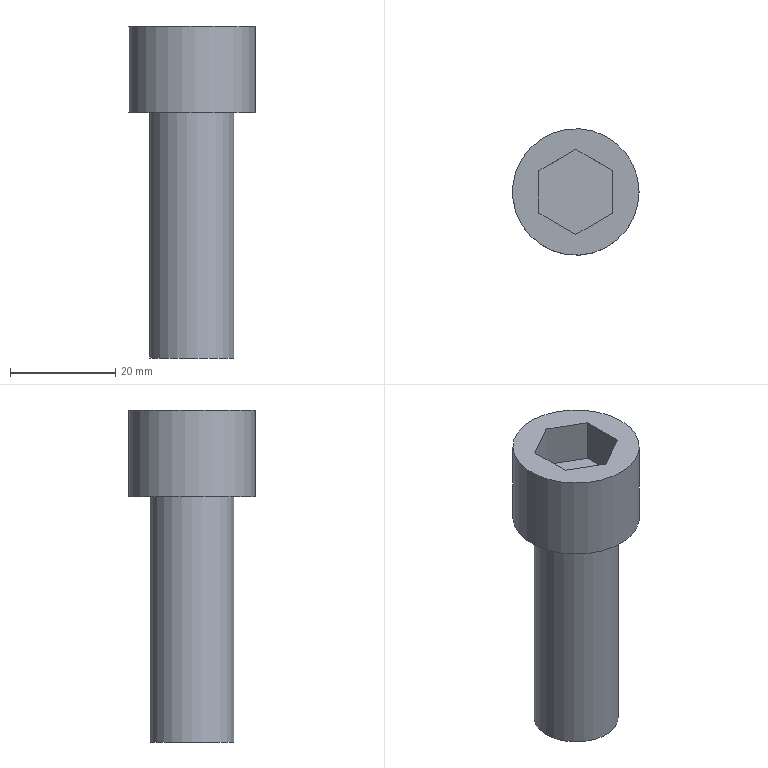Part | NX | features MPPJ 2 | 1 solid | 12 faces | box 24 x 24 x 63 mm | volume 15413 mm3 | plane 10 | cylinder 2 | commonest cylinder face diameters 16 x1 24 x1
STEP:
#1=CARTESIAN_POINT('',(154.5,89.,99.5));
#2=VERTEX_POINT('',#1);
#3=CARTESIAN_POINT('',(142.5,89.,99.5));
#4=DIRECTION('',(0.,0.,-1.));
#5=DIRECTION('',(1.,0.,0.));
#6=AXIS2_PLACEMENT_3D('',#3,#4,#5);
#7=CIRCLE('',#6,12.);
#8=EDGE_CURVE('',#2,#2,#7,.T.);
#9=ORIENTED_EDGE('',*,*,#8,.F.);
#10=EDGE_LOOP('',(#9));
#11=FACE_BOUND('',#10,.T.);
#12=CARTESIAN_POINT('',(149.5,84.959,99.5));
#13=VERTEX_POINT('',#12);
#14=CARTESIAN_POINT('',(142.5,80.917,99.5));
#15=VERTEX_POINT('',#14);
#16=CARTESIAN_POINT('',(149.5,84.959,99.5));
#17=DIRECTION('',(-0.866,-0.5,0.));
#18=VECTOR('',#17,1000.);
#19=LINE('',#16,#18);
#20=EDGE_CURVE('',#13,#15,#19,.T.);
#21=ORIENTED_EDGE('',*,*,#20,.T.);
#22=CARTESIAN_POINT('',(135.5,84.959,99.5));
#23=VERTEX_POINT('',#22);
#24=CARTESIAN_POINT('',(142.5,80.917,99.5));
#25=DIRECTION('',(-0.866,0.5,0.));
#26=VECTOR('',#25,1000.);
#27=LINE('',#24,#26);
#28=EDGE_CURVE('',#15,#23,#27,.T.);
#29=ORIENTED_EDGE('',*,*,#28,.T.);
#30=CARTESIAN_POINT('',(135.5,93.041,99.5));
#31=VERTEX_POINT('',#30);
#32=CARTESIAN_POINT('',(135.5,84.959,99.5));
#33=DIRECTION('',(0.,1.,0.));
#34=VECTOR('',#33,1000.);
#35=LINE('',#32,#34);
#36=EDGE_CURVE('',#23,#31,#35,.T.);
#37=ORIENTED_EDGE('',*,*,#36,.T.);
#38=CARTESIAN_POINT('',(142.5,97.083,99.5));
#39=VERTEX_POINT('',#38);
#40=CARTESIAN_POINT('',(135.5,93.041,99.5));
#41=DIRECTION('',(0.866,0.5,0.));
#42=VECTOR('',#41,1000.);
#43=LINE('',#40,#42);
#44=EDGE_CURVE('',#31,#39,#43,.T.);
#45=ORIENTED_EDGE('',*,*,#44,.T.);
#46=CARTESIAN_POINT('',(149.5,93.041,99.5));
#47=VERTEX_POINT('',#46);
#48=CARTESIAN_POINT('',(142.5,97.083,99.5));
#49=DIRECTION('',(0.866,-0.5,0.));
#50=VECTOR('',#49,1000.);
#51=LINE('',#48,#50);
#52=EDGE_CURVE('',#39,#47,#51,.T.);
#53=ORIENTED_EDGE('',*,*,#52,.T.);
#54=CARTESIAN_POINT('',(149.5,93.041,99.5));
#55=DIRECTION('',(0.,-1.,0.));
#56=VECTOR('',#55,1000.);
#57=LINE('',#54,#56);
#58=EDGE_CURVE('',#47,#13,#57,.T.);
#59=ORIENTED_EDGE('',*,*,#58,.T.);
#60=EDGE_LOOP('',(#21,#29,#37,#45,#53,#59));
#61=FACE_BOUND('',#60,.T.);
#62=CARTESIAN_POINT('',(142.5,89.,99.5));
#63=DIRECTION('',(0.,0.,1.));
#64=DIRECTION('',(1.,0.,0.));
#65=AXIS2_PLACEMENT_3D('',#62,#63,#64);
#66=PLANE('',#65);
#67=ADVANCED_FACE('',(#11,#61),#66,.T.);
#68=CARTESIAN_POINT('',(150.5,89.,36.5));
#69=VERTEX_POINT('',#68);
#70=CARTESIAN_POINT('',(142.5,89.,36.5));
#71=DIRECTION('',(0.,0.,1.));
#72=DIRECTION('',(1.,0.,0.));
#73=AXIS2_PLACEMENT_3D('',#70,#71,#72);
#74=CIRCLE('',#73,8.);
#75=EDGE_CURVE('',#69,#69,#74,.T.);
#76=ORIENTED_EDGE('',*,*,#75,.F.);
#77=EDGE_LOOP('',(#76));
#78=FACE_BOUND('',#77,.T.);
#79=CARTESIAN_POINT('',(142.5,89.,36.5));
#80=DIRECTION('',(0.,0.,-1.));
#81=DIRECTION('',(-1.,0.,0.));
#82=AXIS2_PLACEMENT_3D('',#79,#80,#81);
#83=PLANE('',#82);
#84=ADVANCED_FACE('',(#78),#83,.T.);
#85=CARTESIAN_POINT('',(134.5,89.,83.));
#86=VERTEX_POINT('',#85);
#87=CARTESIAN_POINT('',(142.5,89.,83.));
#88=DIRECTION('',(0.,0.,-1.));
#89=DIRECTION('',(-1.,0.,0.));
#90=AXIS2_PLACEMENT_3D('',#87,#88,#89);
#91=CIRCLE('',#90,8.);
#92=EDGE_CURVE('',#86,#86,#91,.F.);
#93=ORIENTED_EDGE('',*,*,#92,.F.);
#94=EDGE_LOOP('',(#93));
#95=FACE_BOUND('',#94,.T.);
#96=ORIENTED_EDGE('',*,*,#75,.T.);
#97=EDGE_LOOP('',(#96));
#98=FACE_BOUND('',#97,.T.);
#99=CARTESIAN_POINT('',(142.5,89.,99.5));
#100=DIRECTION('',(0.,0.,-1.));
#101=DIRECTION('',(1.,0.,0.));
#102=AXIS2_PLACEMENT_3D('',#99,#100,#101);
#103=CYLINDRICAL_SURFACE('',#102,8.);
#104=ADVANCED_FACE('',(#95,#98),#103,.T.);
#105=ORIENTED_EDGE('',*,*,#92,.T.);
#106=EDGE_LOOP('',(#105));
#107=FACE_BOUND('',#106,.T.);
#108=CARTESIAN_POINT('',(154.5,89.,83.));
#109=VERTEX_POINT('',#108);
#110=CARTESIAN_POINT('',(142.5,89.,83.));
#111=DIRECTION('',(0.,0.,1.));
#112=DIRECTION('',(1.,0.,0.));
#113=AXIS2_PLACEMENT_3D('',#110,#111,#112);
#114=CIRCLE('',#113,12.);
#115=EDGE_CURVE('',#109,#109,#114,.T.);
#116=ORIENTED_EDGE('',*,*,#115,.F.);
#117=EDGE_LOOP('',(#116));
#118=FACE_BOUND('',#117,.T.);
#119=CARTESIAN_POINT('',(142.5,89.,83.));
#120=DIRECTION('',(0.,0.,-1.));
#121=DIRECTION('',(-1.,0.,0.));
#122=AXIS2_PLACEMENT_3D('',#119,#120,#121);
#123=PLANE('',#122);
#124=ADVANCED_FACE('',(#107,#118),#123,.T.);
#125=ORIENTED_EDGE('',*,*,#115,.T.);
#126=EDGE_LOOP('',(#125));
#127=FACE_BOUND('',#126,.T.);
#128=ORIENTED_EDGE('',*,*,#8,.T.);
#129=EDGE_LOOP('',(#128));
#130=FACE_BOUND('',#129,.T.);
#131=CARTESIAN_POINT('',(142.5,89.,99.5));
#132=DIRECTION('',(0.,0.,-1.));
#133=DIRECTION('',(1.,0.,0.));
#134=AXIS2_PLACEMENT_3D('',#131,#132,#133);
#135=CYLINDRICAL_SURFACE('',#134,12.);
#136=ADVANCED_FACE('',(#127,#130),#135,.T.);
#137=CARTESIAN_POINT('',(142.5,80.917,91.25));
#138=VERTEX_POINT('',#137);
#139=CARTESIAN_POINT('',(149.5,84.959,91.25));
#140=VERTEX_POINT('',#139);
#141=CARTESIAN_POINT('',(149.5,84.959,91.25));
#142=DIRECTION('',(-0.866,-0.5,0.));
#143=VECTOR('',#142,1000.);
#144=LINE('',#141,#143);
#145=EDGE_CURVE('',#138,#140,#144,.F.);
#146=ORIENTED_EDGE('',*,*,#145,.F.);
#147=CARTESIAN_POINT('',(142.5,80.917,99.5));
#148=DIRECTION('',(0.,0.,-1.));
#149=VECTOR('',#148,1000.);
#150=LINE('',#147,#149);
#151=EDGE_CURVE('',#138,#15,#150,.F.);
#152=ORIENTED_EDGE('',*,*,#151,.T.);
#153=ORIENTED_EDGE('',*,*,#20,.F.);
#154=CARTESIAN_POINT('',(149.5,84.959,99.5));
#155=DIRECTION('',(0.,0.,-1.));
#156=VECTOR('',#155,1000.);
#157=LINE('',#154,#156);
#158=EDGE_CURVE('',#140,#13,#157,.F.);
#159=ORIENTED_EDGE('',*,*,#158,.F.);
#160=EDGE_LOOP('',(#146,#152,#153,#159));
#161=FACE_BOUND('',#160,.T.);
#162=CARTESIAN_POINT('',(146.,82.938,95.375));
#163=DIRECTION('',(0.5,-0.866,0.));
#164=DIRECTION('',(0.866,0.5,0.));
#165=AXIS2_PLACEMENT_3D('',#162,#163,#164);
#166=PLANE('',#165);
#167=ADVANCED_FACE('',(#161),#166,.F.);
#168=CARTESIAN_POINT('',(149.5,93.041,91.25));
#169=VERTEX_POINT('',#168);
#170=CARTESIAN_POINT('',(149.5,93.041,91.25));
#171=DIRECTION('',(0.,-1.,0.));
#172=VECTOR('',#171,1000.);
#173=LINE('',#170,#172);
#174=EDGE_CURVE('',#140,#169,#173,.F.);
#175=ORIENTED_EDGE('',*,*,#174,.F.);
#176=ORIENTED_EDGE('',*,*,#158,.T.);
#177=ORIENTED_EDGE('',*,*,#58,.F.);
#178=CARTESIAN_POINT('',(149.5,93.041,99.5));
#179=DIRECTION('',(0.,0.,-1.));
#180=VECTOR('',#179,1000.);
#181=LINE('',#178,#180);
#182=EDGE_CURVE('',#169,#47,#181,.F.);
#183=ORIENTED_EDGE('',*,*,#182,.F.);
#184=EDGE_LOOP('',(#175,#176,#177,#183));
#185=FACE_BOUND('',#184,.T.);
#186=CARTESIAN_POINT('',(149.5,89.,95.375));
#187=DIRECTION('',(1.,0.,0.));
#188=DIRECTION('',(0.,0.,-1.));
#189=AXIS2_PLACEMENT_3D('',#186,#187,#188);
#190=PLANE('',#189);
#191=ADVANCED_FACE('',(#185),#190,.F.);
#192=CARTESIAN_POINT('',(142.5,97.083,91.25));
#193=VERTEX_POINT('',#192);
#194=CARTESIAN_POINT('',(142.5,97.083,91.25));
#195=DIRECTION('',(0.866,-0.5,0.));
#196=VECTOR('',#195,1000.);
#197=LINE('',#194,#196);
#198=EDGE_CURVE('',#169,#193,#197,.F.);
#199=ORIENTED_EDGE('',*,*,#198,.F.);
#200=ORIENTED_EDGE('',*,*,#182,.T.);
#201=ORIENTED_EDGE('',*,*,#52,.F.);
#202=CARTESIAN_POINT('',(142.5,97.083,99.5));
#203=DIRECTION('',(0.,0.,-1.));
#204=VECTOR('',#203,1000.);
#205=LINE('',#202,#204);
#206=EDGE_CURVE('',#193,#39,#205,.F.);
#207=ORIENTED_EDGE('',*,*,#206,.F.);
#208=EDGE_LOOP('',(#199,#200,#201,#207));
#209=FACE_BOUND('',#208,.T.);
#210=CARTESIAN_POINT('',(146.,95.062,95.375));
#211=DIRECTION('',(0.5,0.866,0.));
#212=DIRECTION('',(-0.866,0.5,0.));
#213=AXIS2_PLACEMENT_3D('',#210,#211,#212);
#214=PLANE('',#213);
#215=ADVANCED_FACE('',(#209),#214,.F.);
#216=CARTESIAN_POINT('',(135.5,93.041,91.25));
#217=VERTEX_POINT('',#216);
#218=CARTESIAN_POINT('',(135.5,93.041,91.25));
#219=DIRECTION('',(0.866,0.5,0.));
#220=VECTOR('',#219,1000.);
#221=LINE('',#218,#220);
#222=EDGE_CURVE('',#193,#217,#221,.F.);
#223=ORIENTED_EDGE('',*,*,#222,.F.);
#224=ORIENTED_EDGE('',*,*,#206,.T.);
#225=ORIENTED_EDGE('',*,*,#44,.F.);
#226=CARTESIAN_POINT('',(135.5,93.041,99.5));
#227=DIRECTION('',(0.,0.,-1.));
#228=VECTOR('',#227,1000.);
#229=LINE('',#226,#228);
#230=EDGE_CURVE('',#217,#31,#229,.F.);
#231=ORIENTED_EDGE('',*,*,#230,.F.);
#232=EDGE_LOOP('',(#223,#224,#225,#231));
#233=FACE_BOUND('',#232,.T.);
#234=CARTESIAN_POINT('',(139.,95.062,95.375));
#235=DIRECTION('',(-0.5,0.866,0.));
#236=DIRECTION('',(-0.866,-0.5,0.));
#237=AXIS2_PLACEMENT_3D('',#234,#235,#236);
#238=PLANE('',#237);
#239=ADVANCED_FACE('',(#233),#238,.F.);
#240=CARTESIAN_POINT('',(135.5,84.959,91.25));
#241=VERTEX_POINT('',#240);
#242=CARTESIAN_POINT('',(135.5,84.959,91.25));
#243=DIRECTION('',(0.,1.,0.));
#244=VECTOR('',#243,1000.);
#245=LINE('',#242,#244);
#246=EDGE_CURVE('',#217,#241,#245,.F.);
#247=ORIENTED_EDGE('',*,*,#246,.F.);
#248=ORIENTED_EDGE('',*,*,#230,.T.);
#249=ORIENTED_EDGE('',*,*,#36,.F.);
#250=CARTESIAN_POINT('',(135.5,84.959,99.5));
#251=DIRECTION('',(0.,0.,-1.));
#252=VECTOR('',#251,1000.);
#253=LINE('',#250,#252);
#254=EDGE_CURVE('',#241,#23,#253,.F.);
#255=ORIENTED_EDGE('',*,*,#254,.F.);
#256=EDGE_LOOP('',(#247,#248,#249,#255));
#257=FACE_BOUND('',#256,.T.);
#258=CARTESIAN_POINT('',(135.5,89.,95.375));
#259=DIRECTION('',(-1.,0.,0.));
#260=DIRECTION('',(0.,0.,1.));
#261=AXIS2_PLACEMENT_3D('',#258,#259,#260);
#262=PLANE('',#261);
#263=ADVANCED_FACE('',(#257),#262,.F.);
#264=CARTESIAN_POINT('',(142.5,80.917,91.25));
#265=DIRECTION('',(-0.866,0.5,0.));
#266=VECTOR('',#265,1000.);
#267=LINE('',#264,#266);
#268=EDGE_CURVE('',#241,#138,#267,.F.);
#269=ORIENTED_EDGE('',*,*,#268,.F.);
#270=ORIENTED_EDGE('',*,*,#254,.T.);
#271=ORIENTED_EDGE('',*,*,#28,.F.);
#272=ORIENTED_EDGE('',*,*,#151,.F.);
#273=EDGE_LOOP('',(#269,#270,#271,#272));
#274=FACE_BOUND('',#273,.T.);
#275=CARTESIAN_POINT('',(139.,82.938,95.375));
#276=DIRECTION('',(-0.5,-0.866,0.));
#277=DIRECTION('',(0.866,-0.5,0.));
#278=AXIS2_PLACEMENT_3D('',#275,#276,#277);
#279=PLANE('',#278);
#280=ADVANCED_FACE('',(#274),#279,.F.);
#281=ORIENTED_EDGE('',*,*,#174,.T.);
#282=ORIENTED_EDGE('',*,*,#198,.T.);
#283=ORIENTED_EDGE('',*,*,#222,.T.);
#284=ORIENTED_EDGE('',*,*,#246,.T.);
#285=ORIENTED_EDGE('',*,*,#268,.T.);
#286=ORIENTED_EDGE('',*,*,#145,.T.);
#287=EDGE_LOOP('',(#281,#282,#283,#284,#285,#286));
#288=FACE_BOUND('',#287,.T.);
#289=CARTESIAN_POINT('',(142.5,89.,91.25));
#290=DIRECTION('',(0.,0.,-1.));
#291=DIRECTION('',(-1.,0.,0.));
#292=AXIS2_PLACEMENT_3D('',#289,#290,#291);
#293=PLANE('',#292);
#294=ADVANCED_FACE('',(#288),#293,.F.);
#295=CLOSED_SHELL('',(#67,#84,#104,#124,#136,#167,#191,#215,#239,#263,#280,#294));
#296=MANIFOLD_SOLID_BREP('',#295);
#297=(LENGTH_UNIT()NAMED_UNIT(*)SI_UNIT(.MILLI.,.METRE.));
#298=UNCERTAINTY_MEASURE_WITH_UNIT(LENGTH_MEASURE(0.00001),#297,'','');
#299=(NAMED_UNIT(*)PLANE_ANGLE_UNIT()SI_UNIT($,.RADIAN.));
#300=(NAMED_UNIT(*)SI_UNIT($,.STERADIAN.)SOLID_ANGLE_UNIT());
#301=(GEOMETRIC_REPRESENTATION_CONTEXT(3)GLOBAL_UNCERTAINTY_ASSIGNED_CONTEXT((#298))GLOBAL_UNIT_ASSIGNED_CONTEXT((#297,#299,#300))REPRESENTATION_CONTEXT('',''));
#302=ADVANCED_BREP_SHAPE_REPRESENTATION('',(#296),#301);